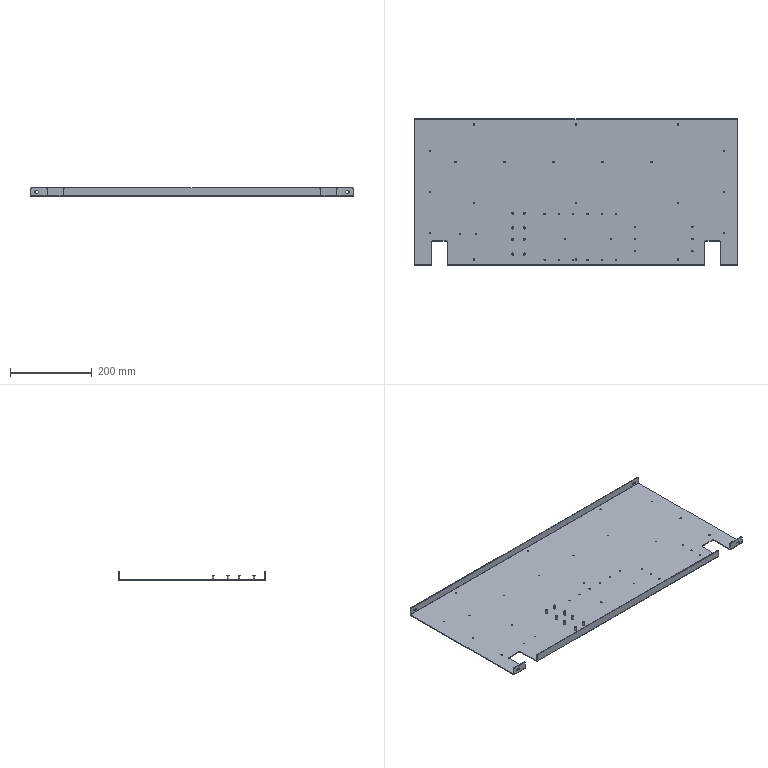Part | STEP file | Electrical mounting plate | 1 solid | 206 faces | box 790 x 360 x 20 mm | volume 612037 mm3 | cylinder 144 | plane 46 | cone 16 | commonest cylinder face diameters 3.3 x80 2.5 x20 5.4 x16 6 x12 5 x8 0.02 x4